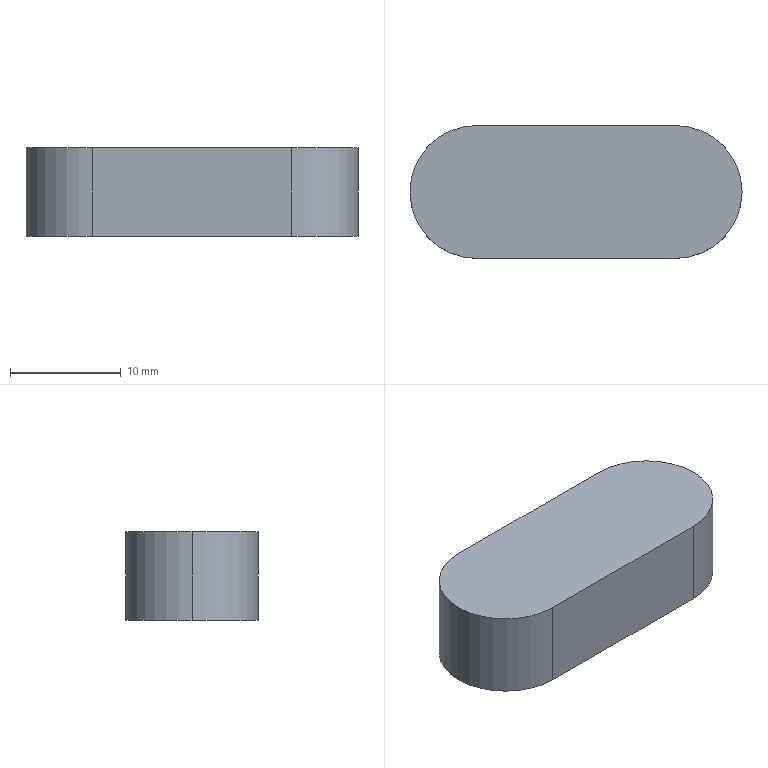Part | SolidWorks | features Extrusion 1, Fillet 1 | 1 solid | 8 faces | box 30 x 12 x 8 mm | volume 2633 mm3 | plane 4 | cylinder 4 | commonest cylinder face diameters 12 x4
STEP:
#1=CARTESIAN_POINT('',(9.,6.,8.));
#2=VERTEX_POINT('',#1);
#3=CARTESIAN_POINT('',(-9.,6.,8.));
#4=VERTEX_POINT('',#3);
#5=CARTESIAN_POINT('',(-15.,6.,8.));
#6=DIRECTION('',(-1.,0.,0.));
#7=VECTOR('',#6,1000.);
#8=LINE('',#5,#7);
#9=EDGE_CURVE('',#2,#4,#8,.T.);
#10=ORIENTED_EDGE('',*,*,#9,.F.);
#11=CARTESIAN_POINT('',(9.,6.,0.));
#12=VERTEX_POINT('',#11);
#13=CARTESIAN_POINT('',(9.,6.,8.));
#14=DIRECTION('',(0.,0.,-1.));
#15=VECTOR('',#14,1000.);
#16=LINE('',#13,#15);
#17=EDGE_CURVE('',#2,#12,#16,.T.);
#18=ORIENTED_EDGE('',*,*,#17,.T.);
#19=CARTESIAN_POINT('',(-9.,6.,0.));
#20=VERTEX_POINT('',#19);
#21=CARTESIAN_POINT('',(-15.,6.,0.));
#22=DIRECTION('',(-1.,0.,0.));
#23=VECTOR('',#22,1000.);
#24=LINE('',#21,#23);
#25=EDGE_CURVE('',#12,#20,#24,.T.);
#26=ORIENTED_EDGE('',*,*,#25,.T.);
#27=CARTESIAN_POINT('',(-9.,6.,8.));
#28=DIRECTION('',(0.,0.,1.));
#29=VECTOR('',#28,1000.);
#30=LINE('',#27,#29);
#31=EDGE_CURVE('',#20,#4,#30,.T.);
#32=ORIENTED_EDGE('',*,*,#31,.T.);
#33=EDGE_LOOP('',(#10,#18,#26,#32));
#34=FACE_OUTER_BOUND('',#33,.T.);
#35=CARTESIAN_POINT('',(-15.,6.,8.));
#36=DIRECTION('',(0.,-1.,0.));
#37=DIRECTION('',(0.,0.,-1.));
#38=AXIS2_PLACEMENT_3D('',#35,#36,#37);
#39=PLANE('',#38);
#40=ADVANCED_FACE('',(#34),#39,.F.);
#41=CARTESIAN_POINT('',(-9.,-6.,0.));
#42=VERTEX_POINT('',#41);
#43=CARTESIAN_POINT('',(9.,-6.,0.));
#44=VERTEX_POINT('',#43);
#45=CARTESIAN_POINT('',(-15.,-6.,0.));
#46=DIRECTION('',(1.,0.,0.));
#47=VECTOR('',#46,1000.);
#48=LINE('',#45,#47);
#49=EDGE_CURVE('',#42,#44,#48,.T.);
#50=ORIENTED_EDGE('',*,*,#49,.T.);
#51=CARTESIAN_POINT('',(9.,-6.,8.));
#52=VERTEX_POINT('',#51);
#53=CARTESIAN_POINT('',(9.,-6.,8.));
#54=DIRECTION('',(0.,0.,1.));
#55=VECTOR('',#54,1000.);
#56=LINE('',#53,#55);
#57=EDGE_CURVE('',#44,#52,#56,.T.);
#58=ORIENTED_EDGE('',*,*,#57,.T.);
#59=CARTESIAN_POINT('',(-9.,-6.,8.));
#60=VERTEX_POINT('',#59);
#61=CARTESIAN_POINT('',(-15.,-6.,8.));
#62=DIRECTION('',(1.,0.,0.));
#63=VECTOR('',#62,1000.);
#64=LINE('',#61,#63);
#65=EDGE_CURVE('',#60,#52,#64,.T.);
#66=ORIENTED_EDGE('',*,*,#65,.F.);
#67=CARTESIAN_POINT('',(-9.,-6.,8.));
#68=DIRECTION('',(0.,0.,-1.));
#69=VECTOR('',#68,1000.);
#70=LINE('',#67,#69);
#71=EDGE_CURVE('',#60,#42,#70,.T.);
#72=ORIENTED_EDGE('',*,*,#71,.T.);
#73=EDGE_LOOP('',(#50,#58,#66,#72));
#74=FACE_OUTER_BOUND('',#73,.T.);
#75=CARTESIAN_POINT('',(-15.,-6.,8.));
#76=DIRECTION('',(0.,1.,0.));
#77=DIRECTION('',(0.,0.,1.));
#78=AXIS2_PLACEMENT_3D('',#75,#76,#77);
#79=PLANE('',#78);
#80=ADVANCED_FACE('',(#74),#79,.F.);
#81=CARTESIAN_POINT('',(15.,0.,8.));
#82=VERTEX_POINT('',#81);
#83=CARTESIAN_POINT('',(9.,0.,8.));
#84=DIRECTION('',(0.,0.,1.));
#85=DIRECTION('',(1.,0.,0.));
#86=AXIS2_PLACEMENT_3D('',#83,#84,#85);
#87=CIRCLE('',#86,6.);
#88=EDGE_CURVE('',#52,#82,#87,.T.);
#89=ORIENTED_EDGE('',*,*,#88,.T.);
#90=CARTESIAN_POINT('',(9.,0.,8.));
#91=DIRECTION('',(0.,0.,1.));
#92=DIRECTION('',(1.,0.,0.));
#93=AXIS2_PLACEMENT_3D('',#90,#91,#92);
#94=CIRCLE('',#93,6.);
#95=EDGE_CURVE('',#82,#2,#94,.T.);
#96=ORIENTED_EDGE('',*,*,#95,.T.);
#97=ORIENTED_EDGE('',*,*,#9,.T.);
#98=CARTESIAN_POINT('',(-15.,0.,8.));
#99=VERTEX_POINT('',#98);
#100=CARTESIAN_POINT('',(-9.,0.,8.));
#101=DIRECTION('',(0.,0.,1.));
#102=DIRECTION('',(1.,0.,0.));
#103=AXIS2_PLACEMENT_3D('',#100,#101,#102);
#104=CIRCLE('',#103,6.);
#105=EDGE_CURVE('',#4,#99,#104,.T.);
#106=ORIENTED_EDGE('',*,*,#105,.T.);
#107=CARTESIAN_POINT('',(-9.,0.,8.));
#108=DIRECTION('',(0.,0.,1.));
#109=DIRECTION('',(1.,0.,0.));
#110=AXIS2_PLACEMENT_3D('',#107,#108,#109);
#111=CIRCLE('',#110,6.);
#112=EDGE_CURVE('',#99,#60,#111,.T.);
#113=ORIENTED_EDGE('',*,*,#112,.T.);
#114=ORIENTED_EDGE('',*,*,#65,.T.);
#115=EDGE_LOOP('',(#89,#96,#97,#106,#113,#114));
#116=FACE_OUTER_BOUND('',#115,.T.);
#117=CARTESIAN_POINT('',(0.,0.,8.));
#118=DIRECTION('',(0.,0.,1.));
#119=DIRECTION('',(1.,0.,0.));
#120=AXIS2_PLACEMENT_3D('',#117,#118,#119);
#121=PLANE('',#120);
#122=ADVANCED_FACE('',(#116),#121,.T.);
#123=ORIENTED_EDGE('',*,*,#25,.F.);
#124=CARTESIAN_POINT('',(15.,0.,0.));
#125=VERTEX_POINT('',#124);
#126=CARTESIAN_POINT('',(9.,0.,0.));
#127=DIRECTION('',(0.,0.,-1.));
#128=DIRECTION('',(1.,0.,0.));
#129=AXIS2_PLACEMENT_3D('',#126,#127,#128);
#130=CIRCLE('',#129,6.);
#131=EDGE_CURVE('',#12,#125,#130,.T.);
#132=ORIENTED_EDGE('',*,*,#131,.T.);
#133=CARTESIAN_POINT('',(9.,0.,0.));
#134=DIRECTION('',(0.,0.,-1.));
#135=DIRECTION('',(1.,0.,0.));
#136=AXIS2_PLACEMENT_3D('',#133,#134,#135);
#137=CIRCLE('',#136,6.);
#138=EDGE_CURVE('',#125,#44,#137,.T.);
#139=ORIENTED_EDGE('',*,*,#138,.T.);
#140=ORIENTED_EDGE('',*,*,#49,.F.);
#141=CARTESIAN_POINT('',(-15.,0.,0.));
#142=VERTEX_POINT('',#141);
#143=CARTESIAN_POINT('',(-9.,0.,0.));
#144=DIRECTION('',(0.,0.,-1.));
#145=DIRECTION('',(1.,0.,0.));
#146=AXIS2_PLACEMENT_3D('',#143,#144,#145);
#147=CIRCLE('',#146,6.);
#148=EDGE_CURVE('',#42,#142,#147,.T.);
#149=ORIENTED_EDGE('',*,*,#148,.T.);
#150=CARTESIAN_POINT('',(-9.,0.,0.));
#151=DIRECTION('',(0.,0.,-1.));
#152=DIRECTION('',(1.,0.,0.));
#153=AXIS2_PLACEMENT_3D('',#150,#151,#152);
#154=CIRCLE('',#153,6.);
#155=EDGE_CURVE('',#142,#20,#154,.T.);
#156=ORIENTED_EDGE('',*,*,#155,.T.);
#157=EDGE_LOOP('',(#123,#132,#139,#140,#149,#156));
#158=FACE_OUTER_BOUND('',#157,.T.);
#159=CARTESIAN_POINT('',(0.,0.,0.));
#160=DIRECTION('',(0.,0.,1.));
#161=DIRECTION('',(1.,0.,0.));
#162=AXIS2_PLACEMENT_3D('',#159,#160,#161);
#163=PLANE('',#162);
#164=ADVANCED_FACE('',(#158),#163,.F.);
#165=CARTESIAN_POINT('',(15.,0.,8.));
#166=DIRECTION('',(0.,0.,-1.));
#167=VECTOR('',#166,1000.);
#168=LINE('',#165,#167);
#169=EDGE_CURVE('',#82,#125,#168,.T.);
#170=ORIENTED_EDGE('',*,*,#169,.F.);
#171=ORIENTED_EDGE('',*,*,#88,.F.);
#172=ORIENTED_EDGE('',*,*,#57,.F.);
#173=ORIENTED_EDGE('',*,*,#138,.F.);
#174=EDGE_LOOP('',(#170,#171,#172,#173));
#175=FACE_OUTER_BOUND('',#174,.T.);
#176=CARTESIAN_POINT('',(9.,0.,8.));
#177=DIRECTION('',(0.,0.,-1.));
#178=DIRECTION('',(-1.,0.,0.));
#179=AXIS2_PLACEMENT_3D('',#176,#177,#178);
#180=CYLINDRICAL_SURFACE('',#179,6.);
#181=ADVANCED_FACE('',(#175),#180,.T.);
#182=ORIENTED_EDGE('',*,*,#95,.F.);
#183=ORIENTED_EDGE('',*,*,#169,.T.);
#184=ORIENTED_EDGE('',*,*,#131,.F.);
#185=ORIENTED_EDGE('',*,*,#17,.F.);
#186=EDGE_LOOP('',(#182,#183,#184,#185));
#187=FACE_OUTER_BOUND('',#186,.T.);
#188=CARTESIAN_POINT('',(9.,0.,8.));
#189=DIRECTION('',(0.,0.,-1.));
#190=DIRECTION('',(-1.,0.,0.));
#191=AXIS2_PLACEMENT_3D('',#188,#189,#190);
#192=CYLINDRICAL_SURFACE('',#191,6.);
#193=ADVANCED_FACE('',(#187),#192,.T.);
#194=CARTESIAN_POINT('',(-15.,0.,8.));
#195=DIRECTION('',(0.,0.,-1.));
#196=VECTOR('',#195,1000.);
#197=LINE('',#194,#196);
#198=EDGE_CURVE('',#99,#142,#197,.T.);
#199=ORIENTED_EDGE('',*,*,#198,.F.);
#200=ORIENTED_EDGE('',*,*,#105,.F.);
#201=ORIENTED_EDGE('',*,*,#31,.F.);
#202=ORIENTED_EDGE('',*,*,#155,.F.);
#203=EDGE_LOOP('',(#199,#200,#201,#202));
#204=FACE_OUTER_BOUND('',#203,.T.);
#205=CARTESIAN_POINT('',(-9.,0.,8.));
#206=DIRECTION('',(0.,0.,-1.));
#207=DIRECTION('',(-1.,0.,0.));
#208=AXIS2_PLACEMENT_3D('',#205,#206,#207);
#209=CYLINDRICAL_SURFACE('',#208,6.);
#210=ADVANCED_FACE('',(#204),#209,.T.);
#211=ORIENTED_EDGE('',*,*,#112,.F.);
#212=ORIENTED_EDGE('',*,*,#198,.T.);
#213=ORIENTED_EDGE('',*,*,#148,.F.);
#214=ORIENTED_EDGE('',*,*,#71,.F.);
#215=EDGE_LOOP('',(#211,#212,#213,#214));
#216=FACE_OUTER_BOUND('',#215,.T.);
#217=CARTESIAN_POINT('',(-9.,0.,8.));
#218=DIRECTION('',(0.,0.,-1.));
#219=DIRECTION('',(-1.,0.,0.));
#220=AXIS2_PLACEMENT_3D('',#217,#218,#219);
#221=CYLINDRICAL_SURFACE('',#220,6.);
#222=ADVANCED_FACE('',(#216),#221,.T.);
#223=CLOSED_SHELL('',(#40,#80,#122,#164,#181,#193,#210,#222));
#224=MANIFOLD_SOLID_BREP('',#223);
#225=CARTESIAN_POINT('',(0.,0.,0.));
#226=DIRECTION('',(0.,0.,1.));
#227=DIRECTION('',(1.,0.,0.));
#228=AXIS2_PLACEMENT_3D('',#225,#226,#227);
#229=(LENGTH_UNIT()NAMED_UNIT(*)SI_UNIT(.MILLI.,.METRE.));
#230=UNCERTAINTY_MEASURE_WITH_UNIT(LENGTH_MEASURE(0.00001),#229,'','');
#231=(NAMED_UNIT(*)PLANE_ANGLE_UNIT()SI_UNIT($,.RADIAN.));
#232=(NAMED_UNIT(*)SI_UNIT($,.STERADIAN.)SOLID_ANGLE_UNIT());
#233=(GEOMETRIC_REPRESENTATION_CONTEXT(3)GLOBAL_UNCERTAINTY_ASSIGNED_CONTEXT((#230))GLOBAL_UNIT_ASSIGNED_CONTEXT((#229,#231,#232))REPRESENTATION_CONTEXT('',''));
#234=ADVANCED_BREP_SHAPE_REPRESENTATION('',(#224,#228),#233);